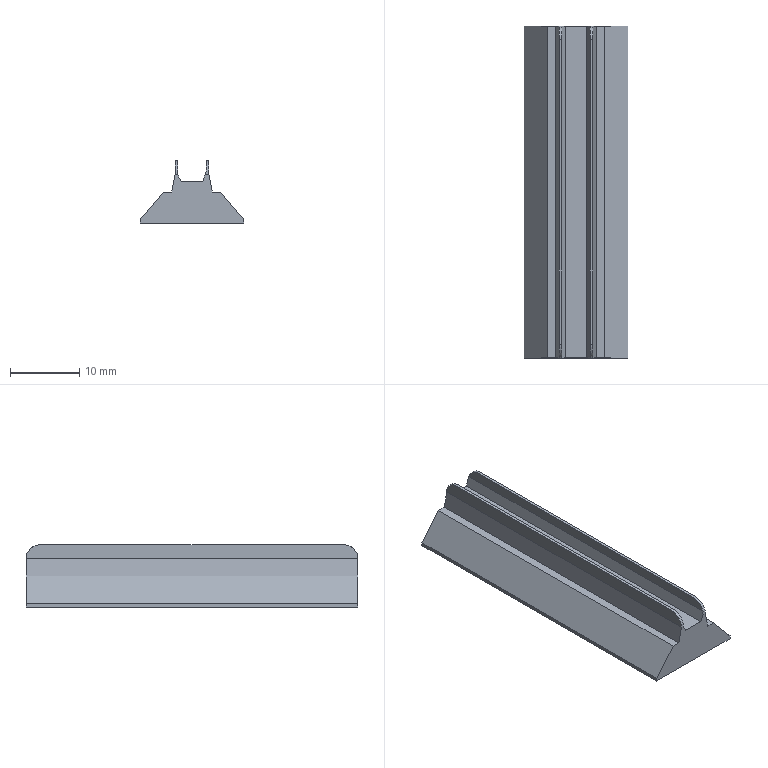Part | SolidWorks | features Chamfer 6, Extrusion 1, Fillet 1 | 1 solid | 24 faces | box 15 x 48 x 9 mm | volume 3152 mm3 | plane 20 | cylinder 4 | commonest cylinder face diameters 4 x4
STEP:
#1=CARTESIAN_POINT('',(2.95,0.,2.25));
#2=VERTEX_POINT('',#1);
#3=CARTESIAN_POINT('',(4.144,0.,2.25));
#4=VERTEX_POINT('',#3);
#5=CARTESIAN_POINT('',(2.45,0.,2.25));
#6=DIRECTION('',(1.,0.,0.));
#7=VECTOR('',#6,1000.);
#8=LINE('',#5,#7);
#9=EDGE_CURVE('',#2,#4,#8,.T.);
#10=ORIENTED_EDGE('',*,*,#9,.T.);
#11=CARTESIAN_POINT('',(4.144,48.,2.25));
#12=VERTEX_POINT('',#11);
#13=CARTESIAN_POINT('',(4.144,48.,2.25));
#14=DIRECTION('',(0.,1.,0.));
#15=VECTOR('',#14,1000.);
#16=LINE('',#13,#15);
#17=EDGE_CURVE('',#4,#12,#16,.T.);
#18=ORIENTED_EDGE('',*,*,#17,.T.);
#19=CARTESIAN_POINT('',(2.95,48.,2.25));
#20=VERTEX_POINT('',#19);
#21=CARTESIAN_POINT('',(2.45,48.,2.25));
#22=DIRECTION('',(1.,0.,0.));
#23=VECTOR('',#22,1000.);
#24=LINE('',#21,#23);
#25=EDGE_CURVE('',#20,#12,#24,.T.);
#26=ORIENTED_EDGE('',*,*,#25,.F.);
#27=CARTESIAN_POINT('',(2.95,0.,2.25));
#28=DIRECTION('',(0.,-1.,0.));
#29=VECTOR('',#28,1000.);
#30=LINE('',#27,#29);
#31=EDGE_CURVE('',#20,#2,#30,.T.);
#32=ORIENTED_EDGE('',*,*,#31,.T.);
#33=EDGE_LOOP('',(#10,#18,#26,#32));
#34=FACE_OUTER_BOUND('',#33,.T.);
#35=CARTESIAN_POINT('',(2.45,48.,2.25));
#36=DIRECTION('',(0.,0.,-1.));
#37=DIRECTION('',(-1.,0.,0.));
#38=AXIS2_PLACEMENT_3D('',#35,#36,#37);
#39=PLANE('',#38);
#40=ADVANCED_FACE('',(#34),#39,.F.);
#41=CARTESIAN_POINT('',(7.5,48.,-1.75));
#42=VERTEX_POINT('',#41);
#43=CARTESIAN_POINT('',(7.5,48.,-2.25));
#44=VERTEX_POINT('',#43);
#45=CARTESIAN_POINT('',(7.5,48.,-2.25));
#46=DIRECTION('',(0.,0.,-1.));
#47=VECTOR('',#46,1000.);
#48=LINE('',#45,#47);
#49=EDGE_CURVE('',#42,#44,#48,.T.);
#50=ORIENTED_EDGE('',*,*,#49,.F.);
#51=CARTESIAN_POINT('',(7.5,0.,-1.75));
#52=VERTEX_POINT('',#51);
#53=CARTESIAN_POINT('',(7.5,48.,-1.75));
#54=DIRECTION('',(0.,-1.,0.));
#55=VECTOR('',#54,1000.);
#56=LINE('',#53,#55);
#57=EDGE_CURVE('',#42,#52,#56,.T.);
#58=ORIENTED_EDGE('',*,*,#57,.T.);
#59=CARTESIAN_POINT('',(7.5,0.,-2.25));
#60=VERTEX_POINT('',#59);
#61=CARTESIAN_POINT('',(7.5,0.,-2.25));
#62=DIRECTION('',(0.,0.,-1.));
#63=VECTOR('',#62,1000.);
#64=LINE('',#61,#63);
#65=EDGE_CURVE('',#52,#60,#64,.T.);
#66=ORIENTED_EDGE('',*,*,#65,.T.);
#67=CARTESIAN_POINT('',(7.5,48.,-2.25));
#68=DIRECTION('',(0.,-1.,0.));
#69=VECTOR('',#68,1000.);
#70=LINE('',#67,#69);
#71=EDGE_CURVE('',#44,#60,#70,.T.);
#72=ORIENTED_EDGE('',*,*,#71,.F.);
#73=EDGE_LOOP('',(#50,#58,#66,#72));
#74=FACE_OUTER_BOUND('',#73,.T.);
#75=CARTESIAN_POINT('',(7.5,48.,-2.25));
#76=DIRECTION('',(-1.,0.,0.));
#77=DIRECTION('',(0.,0.,1.));
#78=AXIS2_PLACEMENT_3D('',#75,#76,#77);
#79=PLANE('',#78);
#80=ADVANCED_FACE('',(#74),#79,.F.);
#81=CARTESIAN_POINT('',(-7.5,0.,-2.25));
#82=VERTEX_POINT('',#81);
#83=CARTESIAN_POINT('',(-7.5,0.,-2.25));
#84=DIRECTION('',(-1.,0.,0.));
#85=VECTOR('',#84,1000.);
#86=LINE('',#83,#85);
#87=EDGE_CURVE('',#60,#82,#86,.T.);
#88=ORIENTED_EDGE('',*,*,#87,.T.);
#89=CARTESIAN_POINT('',(-7.5,48.,-2.25));
#90=VERTEX_POINT('',#89);
#91=CARTESIAN_POINT('',(-7.5,48.,-2.25));
#92=DIRECTION('',(0.,-1.,0.));
#93=VECTOR('',#92,1000.);
#94=LINE('',#91,#93);
#95=EDGE_CURVE('',#90,#82,#94,.T.);
#96=ORIENTED_EDGE('',*,*,#95,.F.);
#97=CARTESIAN_POINT('',(-7.5,48.,-2.25));
#98=DIRECTION('',(-1.,0.,0.));
#99=VECTOR('',#98,1000.);
#100=LINE('',#97,#99);
#101=EDGE_CURVE('',#44,#90,#100,.T.);
#102=ORIENTED_EDGE('',*,*,#101,.F.);
#103=ORIENTED_EDGE('',*,*,#71,.T.);
#104=EDGE_LOOP('',(#88,#96,#102,#103));
#105=FACE_OUTER_BOUND('',#104,.T.);
#106=CARTESIAN_POINT('',(-7.5,48.,-2.25));
#107=DIRECTION('',(0.,0.,1.));
#108=DIRECTION('',(1.,0.,0.));
#109=AXIS2_PLACEMENT_3D('',#106,#107,#108);
#110=PLANE('',#109);
#111=ADVANCED_FACE('',(#105),#110,.F.);
#112=CARTESIAN_POINT('',(-7.5,0.,-1.75));
#113=VERTEX_POINT('',#112);
#114=CARTESIAN_POINT('',(-7.5,0.,-2.25));
#115=DIRECTION('',(0.,0.,1.));
#116=VECTOR('',#115,1000.);
#117=LINE('',#114,#116);
#118=EDGE_CURVE('',#82,#113,#117,.T.);
#119=ORIENTED_EDGE('',*,*,#118,.T.);
#120=CARTESIAN_POINT('',(-7.5,48.,-1.75));
#121=VERTEX_POINT('',#120);
#122=CARTESIAN_POINT('',(-7.5,48.,-1.75));
#123=DIRECTION('',(0.,1.,0.));
#124=VECTOR('',#123,1000.);
#125=LINE('',#122,#124);
#126=EDGE_CURVE('',#113,#121,#125,.T.);
#127=ORIENTED_EDGE('',*,*,#126,.T.);
#128=CARTESIAN_POINT('',(-7.5,48.,-2.25));
#129=DIRECTION('',(0.,0.,1.));
#130=VECTOR('',#129,1000.);
#131=LINE('',#128,#130);
#132=EDGE_CURVE('',#90,#121,#131,.T.);
#133=ORIENTED_EDGE('',*,*,#132,.F.);
#134=ORIENTED_EDGE('',*,*,#95,.T.);
#135=EDGE_LOOP('',(#119,#127,#133,#134));
#136=FACE_OUTER_BOUND('',#135,.T.);
#137=CARTESIAN_POINT('',(-7.5,48.,-2.25));
#138=DIRECTION('',(1.,0.,0.));
#139=DIRECTION('',(0.,0.,-1.));
#140=AXIS2_PLACEMENT_3D('',#137,#138,#139);
#141=PLANE('',#140);
#142=ADVANCED_FACE('',(#136),#141,.F.);
#143=CARTESIAN_POINT('',(-4.144,48.,2.25));
#144=VERTEX_POINT('',#143);
#145=CARTESIAN_POINT('',(-2.95,48.,2.25));
#146=VERTEX_POINT('',#145);
#147=CARTESIAN_POINT('',(-7.5,48.,2.25));
#148=DIRECTION('',(1.,0.,0.));
#149=VECTOR('',#148,1000.);
#150=LINE('',#147,#149);
#151=EDGE_CURVE('',#144,#146,#150,.T.);
#152=ORIENTED_EDGE('',*,*,#151,.F.);
#153=CARTESIAN_POINT('',(-4.144,0.,2.25));
#154=VERTEX_POINT('',#153);
#155=CARTESIAN_POINT('',(-4.144,48.,2.25));
#156=DIRECTION('',(0.,-1.,0.));
#157=VECTOR('',#156,1000.);
#158=LINE('',#155,#157);
#159=EDGE_CURVE('',#144,#154,#158,.T.);
#160=ORIENTED_EDGE('',*,*,#159,.T.);
#161=CARTESIAN_POINT('',(-2.95,0.,2.25));
#162=VERTEX_POINT('',#161);
#163=CARTESIAN_POINT('',(-7.5,0.,2.25));
#164=DIRECTION('',(1.,0.,0.));
#165=VECTOR('',#164,1000.);
#166=LINE('',#163,#165);
#167=EDGE_CURVE('',#154,#162,#166,.T.);
#168=ORIENTED_EDGE('',*,*,#167,.T.);
#169=CARTESIAN_POINT('',(-2.95,48.,2.25));
#170=DIRECTION('',(0.,1.,0.));
#171=VECTOR('',#170,1000.);
#172=LINE('',#169,#171);
#173=EDGE_CURVE('',#162,#146,#172,.T.);
#174=ORIENTED_EDGE('',*,*,#173,.T.);
#175=EDGE_LOOP('',(#152,#160,#168,#174));
#176=FACE_OUTER_BOUND('',#175,.T.);
#177=CARTESIAN_POINT('',(-7.5,48.,2.25));
#178=DIRECTION('',(0.,0.,-1.));
#179=DIRECTION('',(-1.,0.,0.));
#180=AXIS2_PLACEMENT_3D('',#177,#178,#179);
#181=PLANE('',#180);
#182=ADVANCED_FACE('',(#176),#181,.F.);
#183=CARTESIAN_POINT('',(-2.45,48.,4.75));
#184=VERTEX_POINT('',#183);
#185=CARTESIAN_POINT('',(-2.45,0.,4.75));
#186=VERTEX_POINT('',#185);
#187=CARTESIAN_POINT('',(-2.45,0.,4.75));
#188=DIRECTION('',(0.,-1.,0.));
#189=VECTOR('',#188,1000.);
#190=LINE('',#187,#189);
#191=EDGE_CURVE('',#184,#186,#190,.T.);
#192=ORIENTED_EDGE('',*,*,#191,.T.);
#193=CARTESIAN_POINT('',(-2.45,2.,6.75));
#194=VERTEX_POINT('',#193);
#195=CARTESIAN_POINT('',(-2.45,2.,4.75));
#196=DIRECTION('',(-1.,0.,0.));
#197=DIRECTION('',(0.,0.,-1.));
#198=AXIS2_PLACEMENT_3D('',#195,#196,#197);
#199=CIRCLE('',#198,2.);
#200=EDGE_CURVE('',#186,#194,#199,.T.);
#201=ORIENTED_EDGE('',*,*,#200,.T.);
#202=CARTESIAN_POINT('',(-2.45,46.,6.75));
#203=VERTEX_POINT('',#202);
#204=CARTESIAN_POINT('',(-2.45,48.,6.75));
#205=DIRECTION('',(0.,-1.,0.));
#206=VECTOR('',#205,1000.);
#207=LINE('',#204,#206);
#208=EDGE_CURVE('',#203,#194,#207,.T.);
#209=ORIENTED_EDGE('',*,*,#208,.F.);
#210=CARTESIAN_POINT('',(-2.45,46.,4.75));
#211=DIRECTION('',(-1.,0.,0.));
#212=DIRECTION('',(0.,0.,-1.));
#213=AXIS2_PLACEMENT_3D('',#210,#211,#212);
#214=CIRCLE('',#213,2.);
#215=EDGE_CURVE('',#203,#184,#214,.T.);
#216=ORIENTED_EDGE('',*,*,#215,.T.);
#217=EDGE_LOOP('',(#192,#201,#209,#216));
#218=FACE_OUTER_BOUND('',#217,.T.);
#219=CARTESIAN_POINT('',(-2.45,48.,6.75));
#220=DIRECTION('',(1.,0.,0.));
#221=DIRECTION('',(0.,0.,-1.));
#222=AXIS2_PLACEMENT_3D('',#219,#220,#221);
#223=PLANE('',#222);
#224=ADVANCED_FACE('',(#218),#223,.F.);
#225=ORIENTED_EDGE('',*,*,#208,.T.);
#226=CARTESIAN_POINT('',(-2.05,2.,6.75));
#227=VERTEX_POINT('',#226);
#228=CARTESIAN_POINT('',(-2.05,2.,6.75));
#229=DIRECTION('',(1.,0.,0.));
#230=VECTOR('',#229,1000.);
#231=LINE('',#228,#230);
#232=EDGE_CURVE('',#194,#227,#231,.T.);
#233=ORIENTED_EDGE('',*,*,#232,.T.);
#234=CARTESIAN_POINT('',(-2.05,46.,6.75));
#235=VERTEX_POINT('',#234);
#236=CARTESIAN_POINT('',(-2.05,48.,6.75));
#237=DIRECTION('',(0.,-1.,0.));
#238=VECTOR('',#237,1000.);
#239=LINE('',#236,#238);
#240=EDGE_CURVE('',#235,#227,#239,.T.);
#241=ORIENTED_EDGE('',*,*,#240,.F.);
#242=CARTESIAN_POINT('',(-2.45,46.,6.75));
#243=DIRECTION('',(-1.,0.,0.));
#244=VECTOR('',#243,1000.);
#245=LINE('',#242,#244);
#246=EDGE_CURVE('',#235,#203,#245,.T.);
#247=ORIENTED_EDGE('',*,*,#246,.T.);
#248=EDGE_LOOP('',(#225,#233,#241,#247));
#249=FACE_OUTER_BOUND('',#248,.T.);
#250=CARTESIAN_POINT('',(-2.45,48.,6.75));
#251=DIRECTION('',(0.,0.,-1.));
#252=DIRECTION('',(-1.,0.,0.));
#253=AXIS2_PLACEMENT_3D('',#250,#251,#252);
#254=PLANE('',#253);
#255=ADVANCED_FACE('',(#249),#254,.F.);
#256=ORIENTED_EDGE('',*,*,#240,.T.);
#257=CARTESIAN_POINT('',(-2.05,0.,4.75));
#258=VERTEX_POINT('',#257);
#259=CARTESIAN_POINT('',(-2.05,2.,4.75));
#260=DIRECTION('',(1.,0.,0.));
#261=DIRECTION('',(0.,0.,1.));
#262=AXIS2_PLACEMENT_3D('',#259,#260,#261);
#263=CIRCLE('',#262,2.);
#264=EDGE_CURVE('',#227,#258,#263,.T.);
#265=ORIENTED_EDGE('',*,*,#264,.T.);
#266=CARTESIAN_POINT('',(-2.05,48.,4.75));
#267=VERTEX_POINT('',#266);
#268=CARTESIAN_POINT('',(-2.05,48.,4.75));
#269=DIRECTION('',(0.,1.,0.));
#270=VECTOR('',#269,1000.);
#271=LINE('',#268,#270);
#272=EDGE_CURVE('',#258,#267,#271,.T.);
#273=ORIENTED_EDGE('',*,*,#272,.T.);
#274=CARTESIAN_POINT('',(-2.05,46.,4.75));
#275=DIRECTION('',(1.,0.,0.));
#276=DIRECTION('',(0.,0.,1.));
#277=AXIS2_PLACEMENT_3D('',#274,#275,#276);
#278=CIRCLE('',#277,2.);
#279=EDGE_CURVE('',#267,#235,#278,.T.);
#280=ORIENTED_EDGE('',*,*,#279,.T.);
#281=EDGE_LOOP('',(#256,#265,#273,#280));
#282=FACE_OUTER_BOUND('',#281,.T.);
#283=CARTESIAN_POINT('',(-2.05,48.,6.75));
#284=DIRECTION('',(-1.,0.,0.));
#285=DIRECTION('',(0.,0.,1.));
#286=AXIS2_PLACEMENT_3D('',#283,#284,#285);
#287=PLANE('',#286);
#288=ADVANCED_FACE('',(#282),#287,.F.);
#289=CARTESIAN_POINT('',(-1.55,0.,3.75));
#290=VERTEX_POINT('',#289);
#291=CARTESIAN_POINT('',(1.55,0.,3.75));
#292=VERTEX_POINT('',#291);
#293=CARTESIAN_POINT('',(-2.05,0.,3.75));
#294=DIRECTION('',(1.,0.,0.));
#295=VECTOR('',#294,1000.);
#296=LINE('',#293,#295);
#297=EDGE_CURVE('',#290,#292,#296,.T.);
#298=ORIENTED_EDGE('',*,*,#297,.T.);
#299=CARTESIAN_POINT('',(1.55,48.,3.75));
#300=VERTEX_POINT('',#299);
#301=CARTESIAN_POINT('',(1.55,48.,3.75));
#302=DIRECTION('',(0.,1.,0.));
#303=VECTOR('',#302,1000.);
#304=LINE('',#301,#303);
#305=EDGE_CURVE('',#292,#300,#304,.T.);
#306=ORIENTED_EDGE('',*,*,#305,.T.);
#307=CARTESIAN_POINT('',(-1.55,48.,3.75));
#308=VERTEX_POINT('',#307);
#309=CARTESIAN_POINT('',(-2.05,48.,3.75));
#310=DIRECTION('',(1.,0.,0.));
#311=VECTOR('',#310,1000.);
#312=LINE('',#309,#311);
#313=EDGE_CURVE('',#308,#300,#312,.T.);
#314=ORIENTED_EDGE('',*,*,#313,.F.);
#315=CARTESIAN_POINT('',(-1.55,0.,3.75));
#316=DIRECTION('',(0.,-1.,0.));
#317=VECTOR('',#316,1000.);
#318=LINE('',#315,#317);
#319=EDGE_CURVE('',#308,#290,#318,.T.);
#320=ORIENTED_EDGE('',*,*,#319,.T.);
#321=EDGE_LOOP('',(#298,#306,#314,#320));
#322=FACE_OUTER_BOUND('',#321,.T.);
#323=CARTESIAN_POINT('',(-2.05,48.,3.75));
#324=DIRECTION('',(0.,0.,-1.));
#325=DIRECTION('',(-1.,0.,0.));
#326=AXIS2_PLACEMENT_3D('',#323,#324,#325);
#327=PLANE('',#326);
#328=ADVANCED_FACE('',(#322),#327,.F.);
#329=CARTESIAN_POINT('',(2.05,47.936,5.25));
#330=VERTEX_POINT('',#329);
#331=CARTESIAN_POINT('',(2.05,0.06351,5.25));
#332=VERTEX_POINT('',#331);
#333=CARTESIAN_POINT('',(2.05,0.,5.25));
#334=DIRECTION('',(0.,-1.,0.));
#335=VECTOR('',#334,1000.);
#336=LINE('',#333,#335);
#337=EDGE_CURVE('',#330,#332,#336,.T.);
#338=ORIENTED_EDGE('',*,*,#337,.T.);
#339=CARTESIAN_POINT('',(2.05,2.,6.75));
#340=VERTEX_POINT('',#339);
#341=CARTESIAN_POINT('',(2.05,2.,4.75));
#342=DIRECTION('',(-1.,0.,0.));
#343=DIRECTION('',(0.,0.,-1.));
#344=AXIS2_PLACEMENT_3D('',#341,#342,#343);
#345=CIRCLE('',#344,2.);
#346=EDGE_CURVE('',#332,#340,#345,.T.);
#347=ORIENTED_EDGE('',*,*,#346,.T.);
#348=CARTESIAN_POINT('',(2.05,46.,6.75));
#349=VERTEX_POINT('',#348);
#350=CARTESIAN_POINT('',(2.05,48.,6.75));
#351=DIRECTION('',(0.,-1.,0.));
#352=VECTOR('',#351,1000.);
#353=LINE('',#350,#352);
#354=EDGE_CURVE('',#349,#340,#353,.T.);
#355=ORIENTED_EDGE('',*,*,#354,.F.);
#356=CARTESIAN_POINT('',(2.05,46.,4.75));
#357=DIRECTION('',(-1.,0.,0.));
#358=DIRECTION('',(0.,0.,-1.));
#359=AXIS2_PLACEMENT_3D('',#356,#357,#358);
#360=CIRCLE('',#359,2.);
#361=EDGE_CURVE('',#349,#330,#360,.T.);
#362=ORIENTED_EDGE('',*,*,#361,.T.);
#363=EDGE_LOOP('',(#338,#347,#355,#362));
#364=FACE_OUTER_BOUND('',#363,.T.);
#365=CARTESIAN_POINT('',(2.05,48.,6.75));
#366=DIRECTION('',(1.,0.,0.));
#367=DIRECTION('',(0.,0.,-1.));
#368=AXIS2_PLACEMENT_3D('',#365,#366,#367);
#369=PLANE('',#368);
#370=ADVANCED_FACE('',(#364),#369,.F.);
#371=ORIENTED_EDGE('',*,*,#354,.T.);
#372=CARTESIAN_POINT('',(2.45,2.,6.75));
#373=VERTEX_POINT('',#372);
#374=CARTESIAN_POINT('',(2.45,2.,6.75));
#375=DIRECTION('',(1.,0.,0.));
#376=VECTOR('',#375,1000.);
#377=LINE('',#374,#376);
#378=EDGE_CURVE('',#340,#373,#377,.T.);
#379=ORIENTED_EDGE('',*,*,#378,.T.);
#380=CARTESIAN_POINT('',(2.45,46.,6.75));
#381=VERTEX_POINT('',#380);
#382=CARTESIAN_POINT('',(2.45,48.,6.75));
#383=DIRECTION('',(0.,-1.,0.));
#384=VECTOR('',#383,1000.);
#385=LINE('',#382,#384);
#386=EDGE_CURVE('',#381,#373,#385,.T.);
#387=ORIENTED_EDGE('',*,*,#386,.F.);
#388=CARTESIAN_POINT('',(2.05,46.,6.75));
#389=DIRECTION('',(-1.,0.,0.));
#390=VECTOR('',#389,1000.);
#391=LINE('',#388,#390);
#392=EDGE_CURVE('',#381,#349,#391,.T.);
#393=ORIENTED_EDGE('',*,*,#392,.T.);
#394=EDGE_LOOP('',(#371,#379,#387,#393));
#395=FACE_OUTER_BOUND('',#394,.T.);
#396=CARTESIAN_POINT('',(2.05,48.,6.75));
#397=DIRECTION('',(0.,0.,-1.));
#398=DIRECTION('',(-1.,0.,0.));
#399=AXIS2_PLACEMENT_3D('',#396,#397,#398);
#400=PLANE('',#399);
#401=ADVANCED_FACE('',(#395),#400,.F.);
#402=ORIENTED_EDGE('',*,*,#386,.T.);
#403=CARTESIAN_POINT('',(2.45,0.,4.75));
#404=VERTEX_POINT('',#403);
#405=CARTESIAN_POINT('',(2.45,2.,4.75));
#406=DIRECTION('',(1.,0.,0.));
#407=DIRECTION('',(0.,0.,1.));
#408=AXIS2_PLACEMENT_3D('',#405,#406,#407);
#409=CIRCLE('',#408,2.);
#410=EDGE_CURVE('',#373,#404,#409,.T.);
#411=ORIENTED_EDGE('',*,*,#410,.T.);
#412=CARTESIAN_POINT('',(2.45,48.,4.75));
#413=VERTEX_POINT('',#412);
#414=CARTESIAN_POINT('',(2.45,48.,4.75));
#415=DIRECTION('',(0.,1.,0.));
#416=VECTOR('',#415,1000.);
#417=LINE('',#414,#416);
#418=EDGE_CURVE('',#404,#413,#417,.T.);
#419=ORIENTED_EDGE('',*,*,#418,.T.);
#420=CARTESIAN_POINT('',(2.45,46.,4.75));
#421=DIRECTION('',(1.,0.,0.));
#422=DIRECTION('',(0.,0.,1.));
#423=AXIS2_PLACEMENT_3D('',#420,#421,#422);
#424=CIRCLE('',#423,2.);
#425=EDGE_CURVE('',#413,#381,#424,.T.);
#426=ORIENTED_EDGE('',*,*,#425,.T.);
#427=EDGE_LOOP('',(#402,#411,#419,#426));
#428=FACE_OUTER_BOUND('',#427,.T.);
#429=CARTESIAN_POINT('',(2.45,48.,6.75));
#430=DIRECTION('',(-1.,0.,0.));
#431=DIRECTION('',(0.,0.,1.));
#432=AXIS2_PLACEMENT_3D('',#429,#430,#431);
#433=PLANE('',#432);
#434=ADVANCED_FACE('',(#428),#433,.F.);
#435=CARTESIAN_POINT('',(-3.269,48.,0.6538));
#436=DIRECTION('',(0.1961,0.,0.9806));
#437=VECTOR('',#436,1000.);
#438=LINE('',#435,#437);
#439=EDGE_CURVE('',#146,#184,#438,.T.);
#440=ORIENTED_EDGE('',*,*,#439,.T.);
#441=CARTESIAN_POINT('',(0.,48.,4.75));
#442=DIRECTION('',(1.,0.,0.));
#443=VECTOR('',#442,1000.);
#444=LINE('',#441,#443);
#445=EDGE_CURVE('',#184,#267,#444,.T.);
#446=ORIENTED_EDGE('',*,*,#445,.T.);
#447=CARTESIAN_POINT('',(0.26,48.,0.13));
#448=DIRECTION('',(0.4472,0.,-0.8944));
#449=VECTOR('',#448,1000.);
#450=LINE('',#447,#449);
#451=EDGE_CURVE('',#267,#308,#450,.T.);
#452=ORIENTED_EDGE('',*,*,#451,.T.);
#453=ORIENTED_EDGE('',*,*,#313,.T.);
#454=CARTESIAN_POINT('',(1.883,48.,4.75));
#455=VERTEX_POINT('',#454);
#456=CARTESIAN_POINT('',(0.27,48.,-0.09));
#457=DIRECTION('',(0.3162,0.,0.9487));
#458=VECTOR('',#457,1000.);
#459=LINE('',#456,#458);
#460=EDGE_CURVE('',#300,#455,#459,.T.);
#461=ORIENTED_EDGE('',*,*,#460,.T.);
#462=CARTESIAN_POINT('',(0.,48.,4.75));
#463=DIRECTION('',(1.,0.,0.));
#464=VECTOR('',#463,1000.);
#465=LINE('',#462,#464);
#466=EDGE_CURVE('',#455,#413,#465,.T.);
#467=ORIENTED_EDGE('',*,*,#466,.T.);
#468=CARTESIAN_POINT('',(3.269,48.,0.6538));
#469=DIRECTION('',(0.1961,0.,-0.9806));
#470=VECTOR('',#469,1000.);
#471=LINE('',#468,#470);
#472=EDGE_CURVE('',#413,#20,#471,.T.);
#473=ORIENTED_EDGE('',*,*,#472,.T.);
#474=ORIENTED_EDGE('',*,*,#25,.T.);
#475=CARTESIAN_POINT('',(7.5,48.,-1.75));
#476=DIRECTION('',(0.6428,0.,-0.766));
#477=VECTOR('',#476,1000.);
#478=LINE('',#475,#477);
#479=EDGE_CURVE('',#12,#42,#478,.T.);
#480=ORIENTED_EDGE('',*,*,#479,.T.);
#481=ORIENTED_EDGE('',*,*,#49,.T.);
#482=ORIENTED_EDGE('',*,*,#101,.T.);
#483=ORIENTED_EDGE('',*,*,#132,.T.);
#484=CARTESIAN_POINT('',(-4.144,48.,2.25));
#485=DIRECTION('',(0.6428,0.,0.766));
#486=VECTOR('',#485,1000.);
#487=LINE('',#484,#486);
#488=EDGE_CURVE('',#121,#144,#487,.T.);
#489=ORIENTED_EDGE('',*,*,#488,.T.);
#490=ORIENTED_EDGE('',*,*,#151,.T.);
#491=EDGE_LOOP('',(#440,#446,#452,#453,#461,#467,#473,#474,#480,#481,#482,#483,#489,#490));
#492=FACE_OUTER_BOUND('',#491,.T.);
#493=CARTESIAN_POINT('',(0.,48.,0.));
#494=DIRECTION('',(0.,-1.,0.));
#495=DIRECTION('',(0.,0.,-1.));
#496=AXIS2_PLACEMENT_3D('',#493,#494,#495);
#497=PLANE('',#496);
#498=ADVANCED_FACE('',(#492),#497,.F.);
#499=CARTESIAN_POINT('',(-1.55,0.,3.75));
#500=DIRECTION('',(-0.4472,0.,0.8944));
#501=VECTOR('',#500,1000.);
#502=LINE('',#499,#501);
#503=EDGE_CURVE('',#290,#258,#502,.T.);
#504=ORIENTED_EDGE('',*,*,#503,.T.);
#505=CARTESIAN_POINT('',(-2.45,0.,4.75));
#506=DIRECTION('',(-1.,0.,0.));
#507=VECTOR('',#506,1000.);
#508=LINE('',#505,#507);
#509=EDGE_CURVE('',#258,#186,#508,.T.);
#510=ORIENTED_EDGE('',*,*,#509,.T.);
#511=CARTESIAN_POINT('',(-2.45,0.,4.75));
#512=DIRECTION('',(-0.1961,0.,-0.9806));
#513=VECTOR('',#512,1000.);
#514=LINE('',#511,#513);
#515=EDGE_CURVE('',#186,#162,#514,.T.);
#516=ORIENTED_EDGE('',*,*,#515,.T.);
#517=ORIENTED_EDGE('',*,*,#167,.F.);
#518=CARTESIAN_POINT('',(-3.539,0.,2.97));
#519=DIRECTION('',(-0.6428,0.,-0.766));
#520=VECTOR('',#519,1000.);
#521=LINE('',#518,#520);
#522=EDGE_CURVE('',#154,#113,#521,.T.);
#523=ORIENTED_EDGE('',*,*,#522,.T.);
#524=ORIENTED_EDGE('',*,*,#118,.F.);
#525=ORIENTED_EDGE('',*,*,#87,.F.);
#526=ORIENTED_EDGE('',*,*,#65,.F.);
#527=CARTESIAN_POINT('',(3.539,0.,2.97));
#528=DIRECTION('',(-0.6428,0.,0.766));
#529=VECTOR('',#528,1000.);
#530=LINE('',#527,#529);
#531=EDGE_CURVE('',#52,#4,#530,.T.);
#532=ORIENTED_EDGE('',*,*,#531,.T.);
#533=ORIENTED_EDGE('',*,*,#9,.F.);
#534=CARTESIAN_POINT('',(2.95,0.,2.25));
#535=DIRECTION('',(-0.1961,0.,0.9806));
#536=VECTOR('',#535,1000.);
#537=LINE('',#534,#536);
#538=EDGE_CURVE('',#2,#404,#537,.T.);
#539=ORIENTED_EDGE('',*,*,#538,.T.);
#540=CARTESIAN_POINT('',(1.883,0.,4.75));
#541=VERTEX_POINT('',#540);
#542=CARTESIAN_POINT('',(2.05,0.,4.75));
#543=DIRECTION('',(-1.,0.,0.));
#544=VECTOR('',#543,1000.);
#545=LINE('',#542,#544);
#546=EDGE_CURVE('',#404,#541,#545,.T.);
#547=ORIENTED_EDGE('',*,*,#546,.T.);
#548=CARTESIAN_POINT('',(2.05,0.,5.25));
#549=DIRECTION('',(-0.3162,0.,-0.9487));
#550=VECTOR('',#549,1000.);
#551=LINE('',#548,#550);
#552=EDGE_CURVE('',#541,#292,#551,.T.);
#553=ORIENTED_EDGE('',*,*,#552,.T.);
#554=ORIENTED_EDGE('',*,*,#297,.F.);
#555=EDGE_LOOP('',(#504,#510,#516,#517,#523,#524,#525,#526,#532,#533,#539,#547,#553,#554));
#556=FACE_OUTER_BOUND('',#555,.T.);
#557=CARTESIAN_POINT('',(0.,0.,0.));
#558=DIRECTION('',(0.,-1.,0.));
#559=DIRECTION('',(0.,0.,-1.));
#560=AXIS2_PLACEMENT_3D('',#557,#558,#559);
#561=PLANE('',#560);
#562=ADVANCED_FACE('',(#556),#561,.T.);
#563=ORIENTED_EDGE('',*,*,#451,.F.);
#564=ORIENTED_EDGE('',*,*,#272,.F.);
#565=ORIENTED_EDGE('',*,*,#503,.F.);
#566=ORIENTED_EDGE('',*,*,#319,.F.);
#567=EDGE_LOOP('',(#563,#564,#565,#566));
#568=FACE_OUTER_BOUND('',#567,.T.);
#569=CARTESIAN_POINT('',(-1.55,48.,3.75));
#570=DIRECTION('',(0.8944,0.,0.4472));
#571=DIRECTION('',(0.,1.,0.));
#572=AXIS2_PLACEMENT_3D('',#569,#570,#571);
#573=PLANE('',#572);
#574=ADVANCED_FACE('',(#568),#573,.T.);
#575=ORIENTED_EDGE('',*,*,#552,.F.);
#576=CARTESIAN_POINT('',(1.883,0.,4.75));
#577=CARTESIAN_POINT('',(1.94,0.,4.919));
#578=CARTESIAN_POINT('',(1.995,0.02128,5.086));
#579=CARTESIAN_POINT('',(2.05,0.06351,5.25));
#580=(BOUNDED_CURVE()B_SPLINE_CURVE(3,(#576,#577,#578,#579),.UNSPECIFIED.,.F.,.F.)B_SPLINE_CURVE_WITH_KNOTS((4,4),(1.571,1.823),.UNSPECIFIED.)CURVE()GEOMETRIC_REPRESENTATION_ITEM()RATIONAL_B_SPLINE_CURVE((1.,0.9947,0.9947,1.))REPRESENTATION_ITEM(''));
#581=EDGE_CURVE('',#541,#332,#580,.T.);
#582=ORIENTED_EDGE('',*,*,#581,.T.);
#583=ORIENTED_EDGE('',*,*,#337,.F.);
#584=CARTESIAN_POINT('',(2.05,47.936,5.25));
#585=CARTESIAN_POINT('',(1.995,47.979,5.086));
#586=CARTESIAN_POINT('',(1.94,48.,4.919));
#587=CARTESIAN_POINT('',(1.883,48.,4.75));
#588=(BOUNDED_CURVE()B_SPLINE_CURVE(3,(#584,#585,#586,#587),.UNSPECIFIED.,.F.,.F.)B_SPLINE_CURVE_WITH_KNOTS((4,4),(1.318,1.571),.UNSPECIFIED.)CURVE()GEOMETRIC_REPRESENTATION_ITEM()RATIONAL_B_SPLINE_CURVE((1.,0.9947,0.9947,1.))REPRESENTATION_ITEM(''));
#589=EDGE_CURVE('',#330,#455,#588,.T.);
#590=ORIENTED_EDGE('',*,*,#589,.T.);
#591=ORIENTED_EDGE('',*,*,#460,.F.);
#592=ORIENTED_EDGE('',*,*,#305,.F.);
#593=EDGE_LOOP('',(#575,#582,#583,#590,#591,#592));
#594=FACE_OUTER_BOUND('',#593,.T.);
#595=CARTESIAN_POINT('',(2.05,48.,5.25));
#596=DIRECTION('',(-0.9487,0.,0.3162));
#597=DIRECTION('',(0.,1.,0.));
#598=AXIS2_PLACEMENT_3D('',#595,#596,#597);
#599=PLANE('',#598);
#600=ADVANCED_FACE('',(#594),#599,.T.);
#601=ORIENTED_EDGE('',*,*,#439,.F.);
#602=ORIENTED_EDGE('',*,*,#173,.F.);
#603=ORIENTED_EDGE('',*,*,#515,.F.);
#604=ORIENTED_EDGE('',*,*,#191,.F.);
#605=EDGE_LOOP('',(#601,#602,#603,#604));
#606=FACE_OUTER_BOUND('',#605,.T.);
#607=CARTESIAN_POINT('',(-2.45,48.,4.75));
#608=DIRECTION('',(-0.9806,0.,0.1961));
#609=DIRECTION('',(0.,1.,0.));
#610=AXIS2_PLACEMENT_3D('',#607,#608,#609);
#611=PLANE('',#610);
#612=ADVANCED_FACE('',(#606),#611,.T.);
#613=ORIENTED_EDGE('',*,*,#472,.F.);
#614=ORIENTED_EDGE('',*,*,#418,.F.);
#615=ORIENTED_EDGE('',*,*,#538,.F.);
#616=ORIENTED_EDGE('',*,*,#31,.F.);
#617=EDGE_LOOP('',(#613,#614,#615,#616));
#618=FACE_OUTER_BOUND('',#617,.T.);
#619=CARTESIAN_POINT('',(2.95,48.,2.25));
#620=DIRECTION('',(0.9806,0.,0.1961));
#621=DIRECTION('',(0.,1.,0.));
#622=AXIS2_PLACEMENT_3D('',#619,#620,#621);
#623=PLANE('',#622);
#624=ADVANCED_FACE('',(#618),#623,.T.);
#625=ORIENTED_EDGE('',*,*,#488,.F.);
#626=ORIENTED_EDGE('',*,*,#126,.F.);
#627=ORIENTED_EDGE('',*,*,#522,.F.);
#628=ORIENTED_EDGE('',*,*,#159,.F.);
#629=EDGE_LOOP('',(#625,#626,#627,#628));
#630=FACE_OUTER_BOUND('',#629,.T.);
#631=CARTESIAN_POINT('',(-4.144,48.,2.25));
#632=DIRECTION('',(0.766,0.,-0.6428));
#633=DIRECTION('',(0.,-1.,0.));
#634=AXIS2_PLACEMENT_3D('',#631,#632,#633);
#635=PLANE('',#634);
#636=ADVANCED_FACE('',(#630),#635,.F.);
#637=ORIENTED_EDGE('',*,*,#479,.F.);
#638=ORIENTED_EDGE('',*,*,#17,.F.);
#639=ORIENTED_EDGE('',*,*,#531,.F.);
#640=ORIENTED_EDGE('',*,*,#57,.F.);
#641=EDGE_LOOP('',(#637,#638,#639,#640));
#642=FACE_OUTER_BOUND('',#641,.T.);
#643=CARTESIAN_POINT('',(7.5,48.,-1.75));
#644=DIRECTION('',(-0.766,0.,-0.6428));
#645=DIRECTION('',(0.,-1.,0.));
#646=AXIS2_PLACEMENT_3D('',#643,#644,#645);
#647=PLANE('',#646);
#648=ADVANCED_FACE('',(#642),#647,.F.);
#649=ORIENTED_EDGE('',*,*,#200,.F.);
#650=ORIENTED_EDGE('',*,*,#509,.F.);
#651=ORIENTED_EDGE('',*,*,#264,.F.);
#652=ORIENTED_EDGE('',*,*,#232,.F.);
#653=EDGE_LOOP('',(#649,#650,#651,#652));
#654=FACE_OUTER_BOUND('',#653,.T.);
#655=CARTESIAN_POINT('',(-2.45,2.,4.75));
#656=DIRECTION('',(-1.,0.,0.));
#657=DIRECTION('',(0.,0.,1.));
#658=AXIS2_PLACEMENT_3D('',#655,#656,#657);
#659=CYLINDRICAL_SURFACE('',#658,2.);
#660=ADVANCED_FACE('',(#654),#659,.T.);
#661=ORIENTED_EDGE('',*,*,#581,.F.);
#662=ORIENTED_EDGE('',*,*,#546,.F.);
#663=ORIENTED_EDGE('',*,*,#410,.F.);
#664=ORIENTED_EDGE('',*,*,#378,.F.);
#665=ORIENTED_EDGE('',*,*,#346,.F.);
#666=EDGE_LOOP('',(#661,#662,#663,#664,#665));
#667=FACE_OUTER_BOUND('',#666,.T.);
#668=CARTESIAN_POINT('',(2.05,2.,4.75));
#669=DIRECTION('',(-1.,0.,0.));
#670=DIRECTION('',(0.,0.,1.));
#671=AXIS2_PLACEMENT_3D('',#668,#669,#670);
#672=CYLINDRICAL_SURFACE('',#671,2.);
#673=ADVANCED_FACE('',(#667),#672,.T.);
#674=ORIENTED_EDGE('',*,*,#215,.F.);
#675=ORIENTED_EDGE('',*,*,#246,.F.);
#676=ORIENTED_EDGE('',*,*,#279,.F.);
#677=ORIENTED_EDGE('',*,*,#445,.F.);
#678=EDGE_LOOP('',(#674,#675,#676,#677));
#679=FACE_OUTER_BOUND('',#678,.T.);
#680=CARTESIAN_POINT('',(0.,46.,4.75));
#681=DIRECTION('',(1.,0.,0.));
#682=DIRECTION('',(0.,0.,-1.));
#683=AXIS2_PLACEMENT_3D('',#680,#681,#682);
#684=CYLINDRICAL_SURFACE('',#683,2.);
#685=ADVANCED_FACE('',(#679),#684,.T.);
#686=ORIENTED_EDGE('',*,*,#361,.F.);
#687=ORIENTED_EDGE('',*,*,#392,.F.);
#688=ORIENTED_EDGE('',*,*,#425,.F.);
#689=ORIENTED_EDGE('',*,*,#466,.F.);
#690=ORIENTED_EDGE('',*,*,#589,.F.);
#691=EDGE_LOOP('',(#686,#687,#688,#689,#690));
#692=FACE_OUTER_BOUND('',#691,.T.);
#693=CARTESIAN_POINT('',(0.,46.,4.75));
#694=DIRECTION('',(1.,0.,0.));
#695=DIRECTION('',(0.,0.,-1.));
#696=AXIS2_PLACEMENT_3D('',#693,#694,#695);
#697=CYLINDRICAL_SURFACE('',#696,2.);
#698=ADVANCED_FACE('',(#692),#697,.T.);
#699=CLOSED_SHELL('',(#40,#80,#111,#142,#182,#224,#255,#288,#328,#370,#401,#434,#498,#562,#574,#600,#612,#624,#636,#648,#660,#673,#685,#698));
#700=MANIFOLD_SOLID_BREP('',#699);
#701=CARTESIAN_POINT('',(0.,0.,0.));
#702=DIRECTION('',(0.,0.,1.));
#703=DIRECTION('',(1.,0.,0.));
#704=AXIS2_PLACEMENT_3D('',#701,#702,#703);
#705=(LENGTH_UNIT()NAMED_UNIT(*)SI_UNIT(.MILLI.,.METRE.));
#706=UNCERTAINTY_MEASURE_WITH_UNIT(LENGTH_MEASURE(0.00001),#705,'','');
#707=(NAMED_UNIT(*)PLANE_ANGLE_UNIT()SI_UNIT($,.RADIAN.));
#708=(NAMED_UNIT(*)SI_UNIT($,.STERADIAN.)SOLID_ANGLE_UNIT());
#709=(GEOMETRIC_REPRESENTATION_CONTEXT(3)GLOBAL_UNCERTAINTY_ASSIGNED_CONTEXT((#706))GLOBAL_UNIT_ASSIGNED_CONTEXT((#705,#707,#708))REPRESENTATION_CONTEXT('',''));
#710=ADVANCED_BREP_SHAPE_REPRESENTATION('',(#700,#704),#709);